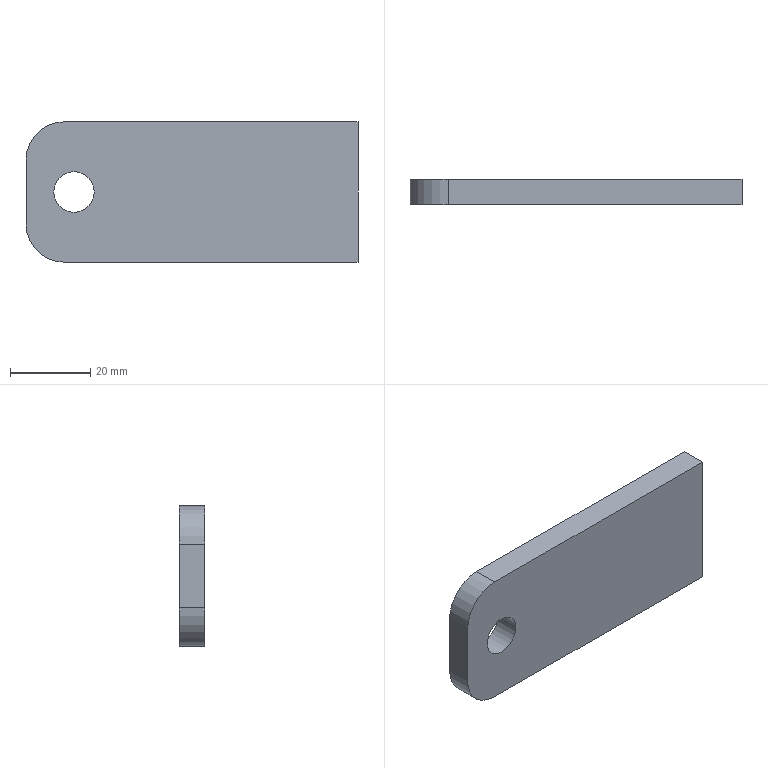Part | NX | features BREP 1 | 1 solid | 10 faces | box 82.55 x 6.35 x 34.925 mm | volume 17558 mm3 | plane 6 | cylinder 4 | commonest cylinder face diameters 10.033 x2 19.05 x2
STEP:
#1=CARTESIAN_POINT('',(0.,0.,-7.938));
#2=VERTEX_POINT('',#1);
#3=CARTESIAN_POINT('',(0.,0.,7.938));
#4=VERTEX_POINT('',#3);
#5=CARTESIAN_POINT('',(0.,0.,-7.938));
#6=DIRECTION('',(0.,0.,1.));
#7=VECTOR('',#6,1000.);
#8=LINE('',#5,#7);
#9=EDGE_CURVE('',#2,#4,#8,.T.);
#10=ORIENTED_EDGE('',*,*,#9,.T.);
#11=CARTESIAN_POINT('',(9.525,0.,17.462));
#12=VERTEX_POINT('',#11);
#13=CARTESIAN_POINT('',(9.525,0.,7.938));
#14=DIRECTION('',(0.,1.,0.));
#15=DIRECTION('',(-1.,0.,0.));
#16=AXIS2_PLACEMENT_3D('',#13,#14,#15);
#17=CIRCLE('',#16,9.525);
#18=EDGE_CURVE('',#4,#12,#17,.T.);
#19=ORIENTED_EDGE('',*,*,#18,.T.);
#20=CARTESIAN_POINT('',(82.55,0.,17.462));
#21=VERTEX_POINT('',#20);
#22=CARTESIAN_POINT('',(9.525,0.,17.462));
#23=DIRECTION('',(1.,0.,0.));
#24=VECTOR('',#23,1000.);
#25=LINE('',#22,#24);
#26=EDGE_CURVE('',#12,#21,#25,.T.);
#27=ORIENTED_EDGE('',*,*,#26,.T.);
#28=CARTESIAN_POINT('',(82.55,0.,-17.462));
#29=VERTEX_POINT('',#28);
#30=CARTESIAN_POINT('',(82.55,0.,17.462));
#31=DIRECTION('',(0.,0.,-1.));
#32=VECTOR('',#31,1000.);
#33=LINE('',#30,#32);
#34=EDGE_CURVE('',#21,#29,#33,.T.);
#35=ORIENTED_EDGE('',*,*,#34,.T.);
#36=CARTESIAN_POINT('',(9.525,0.,-17.462));
#37=VERTEX_POINT('',#36);
#38=CARTESIAN_POINT('',(82.55,0.,-17.462));
#39=DIRECTION('',(-1.,0.,0.));
#40=VECTOR('',#39,1000.);
#41=LINE('',#38,#40);
#42=EDGE_CURVE('',#29,#37,#41,.T.);
#43=ORIENTED_EDGE('',*,*,#42,.T.);
#44=CARTESIAN_POINT('',(9.525,0.,-7.938));
#45=DIRECTION('',(0.,1.,0.));
#46=DIRECTION('',(0.,0.,-1.));
#47=AXIS2_PLACEMENT_3D('',#44,#45,#46);
#48=CIRCLE('',#47,9.525);
#49=EDGE_CURVE('',#37,#2,#48,.T.);
#50=ORIENTED_EDGE('',*,*,#49,.T.);
#51=EDGE_LOOP('',(#10,#19,#27,#35,#43,#50));
#52=FACE_BOUND('',#51,.T.);
#53=CARTESIAN_POINT('',(16.954,0.,0.));
#54=VERTEX_POINT('',#53);
#55=CARTESIAN_POINT('',(6.921,0.,0.));
#56=VERTEX_POINT('',#55);
#57=CARTESIAN_POINT('',(11.938,0.,0.));
#58=DIRECTION('',(0.,1.,0.));
#59=DIRECTION('',(1.,0.,0.));
#60=AXIS2_PLACEMENT_3D('',#57,#58,#59);
#61=CIRCLE('',#60,5.016);
#62=EDGE_CURVE('',#54,#56,#61,.T.);
#63=ORIENTED_EDGE('',*,*,#62,.F.);
#64=CARTESIAN_POINT('',(11.938,0.,0.));
#65=DIRECTION('',(0.,1.,0.));
#66=DIRECTION('',(-1.,0.,0.));
#67=AXIS2_PLACEMENT_3D('',#64,#65,#66);
#68=CIRCLE('',#67,5.016);
#69=EDGE_CURVE('',#56,#54,#68,.T.);
#70=ORIENTED_EDGE('',*,*,#69,.F.);
#71=EDGE_LOOP('',(#63,#70));
#72=FACE_BOUND('',#71,.T.);
#73=CARTESIAN_POINT('',(0.,0.,0.));
#74=DIRECTION('',(0.,1.,0.));
#75=DIRECTION('',(1.,0.,0.));
#76=AXIS2_PLACEMENT_3D('',#73,#74,#75);
#77=PLANE('',#76);
#78=ADVANCED_FACE('',(#52,#72),#77,.T.);
#79=CARTESIAN_POINT('',(16.954,-6.35,0.));
#80=VERTEX_POINT('',#79);
#81=CARTESIAN_POINT('',(16.954,0.,0.));
#82=DIRECTION('',(0.,-1.,0.));
#83=VECTOR('',#82,1000.);
#84=LINE('',#81,#83);
#85=EDGE_CURVE('',#80,#54,#84,.F.);
#86=ORIENTED_EDGE('',*,*,#85,.F.);
#87=CARTESIAN_POINT('',(6.921,-6.35,0.));
#88=VERTEX_POINT('',#87);
#89=CARTESIAN_POINT('',(11.938,-6.35,0.));
#90=DIRECTION('',(0.,1.,0.));
#91=DIRECTION('',(-1.,0.,0.));
#92=AXIS2_PLACEMENT_3D('',#89,#90,#91);
#93=CIRCLE('',#92,5.016);
#94=EDGE_CURVE('',#88,#80,#93,.T.);
#95=ORIENTED_EDGE('',*,*,#94,.F.);
#96=CARTESIAN_POINT('',(6.921,0.,0.));
#97=DIRECTION('',(0.,-1.,0.));
#98=VECTOR('',#97,1000.);
#99=LINE('',#96,#98);
#100=EDGE_CURVE('',#88,#56,#99,.F.);
#101=ORIENTED_EDGE('',*,*,#100,.T.);
#102=ORIENTED_EDGE('',*,*,#69,.T.);
#103=EDGE_LOOP('',(#86,#95,#101,#102));
#104=FACE_BOUND('',#103,.T.);
#105=CARTESIAN_POINT('',(11.938,-3.175,0.));
#106=DIRECTION('',(0.,1.,0.));
#107=DIRECTION('',(-1.,0.,0.));
#108=AXIS2_PLACEMENT_3D('',#105,#106,#107);
#109=CYLINDRICAL_SURFACE('',#108,5.016);
#110=ADVANCED_FACE('',(#104),#109,.F.);
#111=ORIENTED_EDGE('',*,*,#100,.F.);
#112=CARTESIAN_POINT('',(11.938,-6.35,0.));
#113=DIRECTION('',(0.,1.,0.));
#114=DIRECTION('',(1.,0.,0.));
#115=AXIS2_PLACEMENT_3D('',#112,#113,#114);
#116=CIRCLE('',#115,5.016);
#117=EDGE_CURVE('',#80,#88,#116,.T.);
#118=ORIENTED_EDGE('',*,*,#117,.F.);
#119=ORIENTED_EDGE('',*,*,#85,.T.);
#120=ORIENTED_EDGE('',*,*,#62,.T.);
#121=EDGE_LOOP('',(#111,#118,#119,#120));
#122=FACE_BOUND('',#121,.T.);
#123=CARTESIAN_POINT('',(11.938,-3.175,0.));
#124=DIRECTION('',(0.,1.,0.));
#125=DIRECTION('',(1.,0.,0.));
#126=AXIS2_PLACEMENT_3D('',#123,#124,#125);
#127=CYLINDRICAL_SURFACE('',#126,5.016);
#128=ADVANCED_FACE('',(#122),#127,.F.);
#129=CARTESIAN_POINT('',(82.55,-6.35,-17.462));
#130=VERTEX_POINT('',#129);
#131=CARTESIAN_POINT('',(9.525,-6.35,-17.462));
#132=VERTEX_POINT('',#131);
#133=CARTESIAN_POINT('',(82.55,-6.35,-17.462));
#134=DIRECTION('',(-1.,0.,0.));
#135=VECTOR('',#134,1000.);
#136=LINE('',#133,#135);
#137=EDGE_CURVE('',#130,#132,#136,.T.);
#138=ORIENTED_EDGE('',*,*,#137,.F.);
#139=CARTESIAN_POINT('',(82.55,-6.35,17.462));
#140=VERTEX_POINT('',#139);
#141=CARTESIAN_POINT('',(82.55,-6.35,17.462));
#142=DIRECTION('',(0.,0.,-1.));
#143=VECTOR('',#142,1000.);
#144=LINE('',#141,#143);
#145=EDGE_CURVE('',#140,#130,#144,.T.);
#146=ORIENTED_EDGE('',*,*,#145,.F.);
#147=CARTESIAN_POINT('',(9.525,-6.35,17.462));
#148=VERTEX_POINT('',#147);
#149=CARTESIAN_POINT('',(9.525,-6.35,17.462));
#150=DIRECTION('',(1.,0.,0.));
#151=VECTOR('',#150,1000.);
#152=LINE('',#149,#151);
#153=EDGE_CURVE('',#148,#140,#152,.T.);
#154=ORIENTED_EDGE('',*,*,#153,.F.);
#155=CARTESIAN_POINT('',(0.,-6.35,7.938));
#156=VERTEX_POINT('',#155);
#157=CARTESIAN_POINT('',(9.525,-6.35,7.938));
#158=DIRECTION('',(0.,-1.,0.));
#159=DIRECTION('',(0.,0.,1.));
#160=AXIS2_PLACEMENT_3D('',#157,#158,#159);
#161=CIRCLE('',#160,9.525);
#162=EDGE_CURVE('',#148,#156,#161,.T.);
#163=ORIENTED_EDGE('',*,*,#162,.T.);
#164=CARTESIAN_POINT('',(0.,-6.35,-7.938));
#165=VERTEX_POINT('',#164);
#166=CARTESIAN_POINT('',(0.,-6.35,-7.938));
#167=DIRECTION('',(0.,0.,1.));
#168=VECTOR('',#167,1000.);
#169=LINE('',#166,#168);
#170=EDGE_CURVE('',#165,#156,#169,.T.);
#171=ORIENTED_EDGE('',*,*,#170,.F.);
#172=CARTESIAN_POINT('',(9.525,-6.35,-7.938));
#173=DIRECTION('',(0.,-1.,0.));
#174=DIRECTION('',(-1.,0.,0.));
#175=AXIS2_PLACEMENT_3D('',#172,#173,#174);
#176=CIRCLE('',#175,9.525);
#177=EDGE_CURVE('',#165,#132,#176,.T.);
#178=ORIENTED_EDGE('',*,*,#177,.T.);
#179=EDGE_LOOP('',(#138,#146,#154,#163,#171,#178));
#180=FACE_BOUND('',#179,.T.);
#181=ORIENTED_EDGE('',*,*,#117,.T.);
#182=ORIENTED_EDGE('',*,*,#94,.T.);
#183=EDGE_LOOP('',(#181,#182));
#184=FACE_BOUND('',#183,.T.);
#185=CARTESIAN_POINT('',(0.,-6.35,0.));
#186=DIRECTION('',(0.,1.,0.));
#187=DIRECTION('',(1.,0.,0.));
#188=AXIS2_PLACEMENT_3D('',#185,#186,#187);
#189=PLANE('',#188);
#190=ADVANCED_FACE('',(#180,#184),#189,.F.);
#191=ORIENTED_EDGE('',*,*,#177,.F.);
#192=CARTESIAN_POINT('',(0.,-6.35,-7.938));
#193=DIRECTION('',(0.,1.,0.));
#194=VECTOR('',#193,1000.);
#195=LINE('',#192,#194);
#196=EDGE_CURVE('',#165,#2,#195,.T.);
#197=ORIENTED_EDGE('',*,*,#196,.T.);
#198=ORIENTED_EDGE('',*,*,#49,.F.);
#199=CARTESIAN_POINT('',(9.525,-6.35,-17.462));
#200=DIRECTION('',(0.,1.,0.));
#201=VECTOR('',#200,1000.);
#202=LINE('',#199,#201);
#203=EDGE_CURVE('',#132,#37,#202,.T.);
#204=ORIENTED_EDGE('',*,*,#203,.F.);
#205=EDGE_LOOP('',(#191,#197,#198,#204));
#206=FACE_BOUND('',#205,.T.);
#207=CARTESIAN_POINT('',(9.525,-6.48,-7.938));
#208=DIRECTION('',(0.,1.,0.));
#209=DIRECTION('',(0.,0.,-1.));
#210=AXIS2_PLACEMENT_3D('',#207,#208,#209);
#211=CYLINDRICAL_SURFACE('',#210,9.525);
#212=ADVANCED_FACE('',(#206),#211,.T.);
#213=ORIENTED_EDGE('',*,*,#42,.F.);
#214=CARTESIAN_POINT('',(82.55,0.,-17.462));
#215=DIRECTION('',(0.,-1.,0.));
#216=VECTOR('',#215,1000.);
#217=LINE('',#214,#216);
#218=EDGE_CURVE('',#29,#130,#217,.T.);
#219=ORIENTED_EDGE('',*,*,#218,.T.);
#220=ORIENTED_EDGE('',*,*,#137,.T.);
#221=ORIENTED_EDGE('',*,*,#203,.T.);
#222=EDGE_LOOP('',(#213,#219,#220,#221));
#223=FACE_BOUND('',#222,.T.);
#224=CARTESIAN_POINT('',(41.275,-3.175,-17.462));
#225=DIRECTION('',(0.,0.,-1.));
#226=DIRECTION('',(0.,-1.,0.));
#227=AXIS2_PLACEMENT_3D('',#224,#225,#226);
#228=PLANE('',#227);
#229=ADVANCED_FACE('',(#223),#228,.T.);
#230=CARTESIAN_POINT('',(82.55,0.,17.462));
#231=DIRECTION('',(0.,-1.,0.));
#232=VECTOR('',#231,1000.);
#233=LINE('',#230,#232);
#234=EDGE_CURVE('',#21,#140,#233,.T.);
#235=ORIENTED_EDGE('',*,*,#234,.T.);
#236=ORIENTED_EDGE('',*,*,#145,.T.);
#237=ORIENTED_EDGE('',*,*,#218,.F.);
#238=ORIENTED_EDGE('',*,*,#34,.F.);
#239=EDGE_LOOP('',(#235,#236,#237,#238));
#240=FACE_BOUND('',#239,.T.);
#241=CARTESIAN_POINT('',(82.55,-3.175,0.));
#242=DIRECTION('',(1.,0.,0.));
#243=DIRECTION('',(0.,1.,0.));
#244=AXIS2_PLACEMENT_3D('',#241,#242,#243);
#245=PLANE('',#244);
#246=ADVANCED_FACE('',(#240),#245,.T.);
#247=ORIENTED_EDGE('',*,*,#153,.T.);
#248=ORIENTED_EDGE('',*,*,#234,.F.);
#249=ORIENTED_EDGE('',*,*,#26,.F.);
#250=CARTESIAN_POINT('',(9.525,-6.35,17.462));
#251=DIRECTION('',(0.,1.,0.));
#252=VECTOR('',#251,1000.);
#253=LINE('',#250,#252);
#254=EDGE_CURVE('',#148,#12,#253,.T.);
#255=ORIENTED_EDGE('',*,*,#254,.F.);
#256=EDGE_LOOP('',(#247,#248,#249,#255));
#257=FACE_BOUND('',#256,.T.);
#258=CARTESIAN_POINT('',(41.275,-3.175,17.462));
#259=DIRECTION('',(0.,0.,1.));
#260=DIRECTION('',(1.,0.,0.));
#261=AXIS2_PLACEMENT_3D('',#258,#259,#260);
#262=PLANE('',#261);
#263=ADVANCED_FACE('',(#257),#262,.T.);
#264=ORIENTED_EDGE('',*,*,#162,.F.);
#265=ORIENTED_EDGE('',*,*,#254,.T.);
#266=ORIENTED_EDGE('',*,*,#18,.F.);
#267=CARTESIAN_POINT('',(0.,-6.35,7.938));
#268=DIRECTION('',(0.,1.,0.));
#269=VECTOR('',#268,1000.);
#270=LINE('',#267,#269);
#271=EDGE_CURVE('',#156,#4,#270,.T.);
#272=ORIENTED_EDGE('',*,*,#271,.F.);
#273=EDGE_LOOP('',(#264,#265,#266,#272));
#274=FACE_BOUND('',#273,.T.);
#275=CARTESIAN_POINT('',(9.525,-6.48,7.938));
#276=DIRECTION('',(0.,1.,0.));
#277=DIRECTION('',(-1.,0.,0.));
#278=AXIS2_PLACEMENT_3D('',#275,#276,#277);
#279=CYLINDRICAL_SURFACE('',#278,9.525);
#280=ADVANCED_FACE('',(#274),#279,.T.);
#281=ORIENTED_EDGE('',*,*,#170,.T.);
#282=ORIENTED_EDGE('',*,*,#271,.T.);
#283=ORIENTED_EDGE('',*,*,#9,.F.);
#284=ORIENTED_EDGE('',*,*,#196,.F.);
#285=EDGE_LOOP('',(#281,#282,#283,#284));
#286=FACE_BOUND('',#285,.T.);
#287=CARTESIAN_POINT('',(0.,-3.175,0.));
#288=DIRECTION('',(-1.,0.,0.));
#289=DIRECTION('',(0.,0.,1.));
#290=AXIS2_PLACEMENT_3D('',#287,#288,#289);
#291=PLANE('',#290);
#292=ADVANCED_FACE('',(#286),#291,.T.);
#293=CLOSED_SHELL('',(#78,#110,#128,#190,#212,#229,#246,#263,#280,#292));
#294=MANIFOLD_SOLID_BREP('',#293);
#295=(LENGTH_UNIT()NAMED_UNIT(*)SI_UNIT(.MILLI.,.METRE.));
#296=UNCERTAINTY_MEASURE_WITH_UNIT(LENGTH_MEASURE(0.00001),#295,'','');
#297=(NAMED_UNIT(*)PLANE_ANGLE_UNIT()SI_UNIT($,.RADIAN.));
#298=(NAMED_UNIT(*)SI_UNIT($,.STERADIAN.)SOLID_ANGLE_UNIT());
#299=(GEOMETRIC_REPRESENTATION_CONTEXT(3)GLOBAL_UNCERTAINTY_ASSIGNED_CONTEXT((#296))GLOBAL_UNIT_ASSIGNED_CONTEXT((#295,#297,#298))REPRESENTATION_CONTEXT('',''));
#300=ADVANCED_BREP_SHAPE_REPRESENTATION('',(#294),#299);